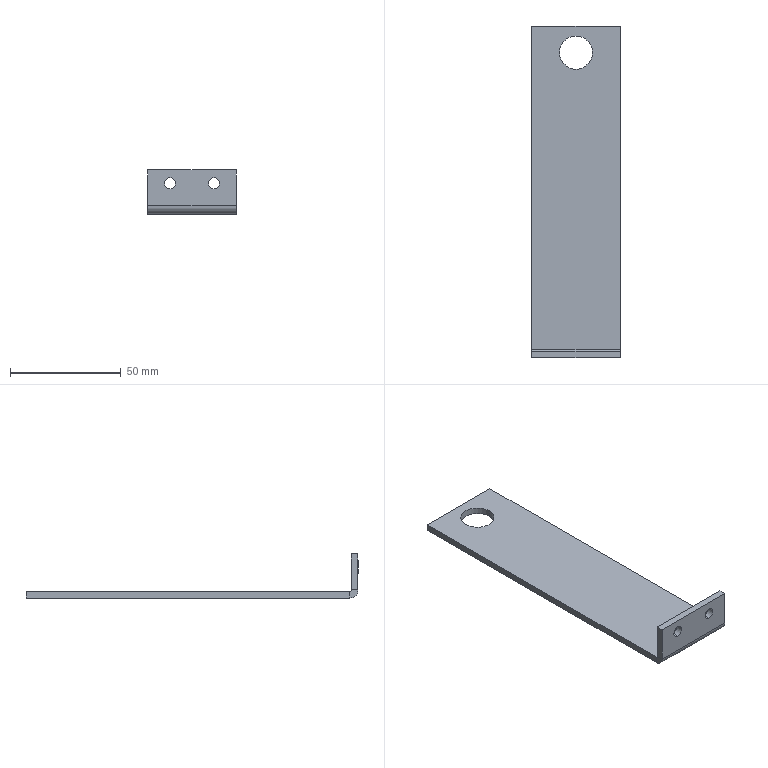Part | SolidWorks | features ICE 2, EdgeFlange 1, FlatPattern 1, SMBaseFlange 1, SheetMetal 1 | 1 solid | 20 faces | box 40 x 150 x 20 mm | volume 19277 mm3 | plane 12 | cylinder 8 | commonest cylinder face diameters 5 x4 15 x2 1.473 x1 7.473 x1
STEP:
#1=CARTESIAN_POINT('',(-10.,-75.,8.5));
#2=VERTEX_POINT('',#1);
#3=CARTESIAN_POINT('',(-10.,-75.,13.5));
#4=VERTEX_POINT('',#3);
#5=CARTESIAN_POINT('',(-10.,-75.,11.));
#6=DIRECTION('',(0.,1.,0.));
#7=DIRECTION('',(0.,0.,1.));
#8=AXIS2_PLACEMENT_3D('',#5,#6,#7);
#9=CIRCLE('',#8,2.5);
#10=EDGE_CURVE('',#2,#4,#9,.T.);
#11=ORIENTED_EDGE('',*,*,#10,.F.);
#12=CARTESIAN_POINT('',(-10.,-72.,8.5));
#13=VERTEX_POINT('',#12);
#14=CARTESIAN_POINT('',(-10.,-75.,8.5));
#15=DIRECTION('',(0.,1.,0.));
#16=VECTOR('',#15,1000.);
#17=LINE('',#14,#16);
#18=EDGE_CURVE('',#2,#13,#17,.T.);
#19=ORIENTED_EDGE('',*,*,#18,.T.);
#20=CARTESIAN_POINT('',(-10.,-72.,13.5));
#21=VERTEX_POINT('',#20);
#22=CARTESIAN_POINT('',(-10.,-72.,11.));
#23=DIRECTION('',(0.,1.,0.));
#24=DIRECTION('',(0.,0.,1.));
#25=AXIS2_PLACEMENT_3D('',#22,#23,#24);
#26=CIRCLE('',#25,2.5);
#27=EDGE_CURVE('',#13,#21,#26,.T.);
#28=ORIENTED_EDGE('',*,*,#27,.T.);
#29=CARTESIAN_POINT('',(-10.,-75.,13.5));
#30=DIRECTION('',(0.,1.,0.));
#31=VECTOR('',#30,1000.);
#32=LINE('',#29,#31);
#33=EDGE_CURVE('',#4,#21,#32,.T.);
#34=ORIENTED_EDGE('',*,*,#33,.F.);
#35=EDGE_LOOP('',(#11,#19,#28,#34));
#36=FACE_OUTER_BOUND('',#35,.T.);
#37=CARTESIAN_POINT('',(-10.,-75.,11.));
#38=DIRECTION('',(0.,1.,0.));
#39=DIRECTION('',(0.,0.,1.));
#40=AXIS2_PLACEMENT_3D('',#37,#38,#39);
#41=CYLINDRICAL_SURFACE('',#40,2.5);
#42=ADVANCED_FACE('',(#36),#41,.F.);
#43=CARTESIAN_POINT('',(10.,-75.,8.5));
#44=VERTEX_POINT('',#43);
#45=CARTESIAN_POINT('',(10.,-75.,13.5));
#46=VERTEX_POINT('',#45);
#47=CARTESIAN_POINT('',(10.,-75.,11.));
#48=DIRECTION('',(0.,1.,0.));
#49=DIRECTION('',(0.,0.,1.));
#50=AXIS2_PLACEMENT_3D('',#47,#48,#49);
#51=CIRCLE('',#50,2.5);
#52=EDGE_CURVE('',#44,#46,#51,.T.);
#53=ORIENTED_EDGE('',*,*,#52,.F.);
#54=CARTESIAN_POINT('',(10.,-72.,8.5));
#55=VERTEX_POINT('',#54);
#56=CARTESIAN_POINT('',(10.,-75.,8.5));
#57=DIRECTION('',(0.,1.,0.));
#58=VECTOR('',#57,1000.);
#59=LINE('',#56,#58);
#60=EDGE_CURVE('',#44,#55,#59,.T.);
#61=ORIENTED_EDGE('',*,*,#60,.T.);
#62=CARTESIAN_POINT('',(10.,-72.,13.5));
#63=VERTEX_POINT('',#62);
#64=CARTESIAN_POINT('',(10.,-72.,11.));
#65=DIRECTION('',(0.,1.,0.));
#66=DIRECTION('',(0.,0.,1.));
#67=AXIS2_PLACEMENT_3D('',#64,#65,#66);
#68=CIRCLE('',#67,2.5);
#69=EDGE_CURVE('',#55,#63,#68,.T.);
#70=ORIENTED_EDGE('',*,*,#69,.T.);
#71=CARTESIAN_POINT('',(10.,-75.,13.5));
#72=DIRECTION('',(0.,1.,0.));
#73=VECTOR('',#72,1000.);
#74=LINE('',#71,#73);
#75=EDGE_CURVE('',#46,#63,#74,.T.);
#76=ORIENTED_EDGE('',*,*,#75,.F.);
#77=EDGE_LOOP('',(#53,#61,#70,#76));
#78=FACE_OUTER_BOUND('',#77,.T.);
#79=CARTESIAN_POINT('',(10.,-75.,11.));
#80=DIRECTION('',(0.,1.,0.));
#81=DIRECTION('',(0.,0.,1.));
#82=AXIS2_PLACEMENT_3D('',#79,#80,#81);
#83=CYLINDRICAL_SURFACE('',#82,2.5);
#84=ADVANCED_FACE('',(#78),#83,.F.);
#85=CARTESIAN_POINT('',(-7.5,63.,-3.));
#86=VERTEX_POINT('',#85);
#87=CARTESIAN_POINT('',(7.5,63.,-3.));
#88=VERTEX_POINT('',#87);
#89=CARTESIAN_POINT('',(0.,63.,-3.));
#90=DIRECTION('',(0.,0.,1.));
#91=DIRECTION('',(1.,0.,0.));
#92=AXIS2_PLACEMENT_3D('',#89,#90,#91);
#93=CIRCLE('',#92,7.5);
#94=EDGE_CURVE('',#86,#88,#93,.T.);
#95=ORIENTED_EDGE('',*,*,#94,.F.);
#96=CARTESIAN_POINT('',(-7.5,63.,0.));
#97=VERTEX_POINT('',#96);
#98=CARTESIAN_POINT('',(-7.5,63.,-3.));
#99=DIRECTION('',(0.,0.,1.));
#100=VECTOR('',#99,1000.);
#101=LINE('',#98,#100);
#102=EDGE_CURVE('',#86,#97,#101,.T.);
#103=ORIENTED_EDGE('',*,*,#102,.T.);
#104=CARTESIAN_POINT('',(7.5,63.,0.));
#105=VERTEX_POINT('',#104);
#106=CARTESIAN_POINT('',(0.,63.,0.));
#107=DIRECTION('',(0.,0.,1.));
#108=DIRECTION('',(1.,0.,0.));
#109=AXIS2_PLACEMENT_3D('',#106,#107,#108);
#110=CIRCLE('',#109,7.5);
#111=EDGE_CURVE('',#97,#105,#110,.T.);
#112=ORIENTED_EDGE('',*,*,#111,.T.);
#113=CARTESIAN_POINT('',(7.5,63.,-3.));
#114=DIRECTION('',(0.,0.,1.));
#115=VECTOR('',#114,1000.);
#116=LINE('',#113,#115);
#117=EDGE_CURVE('',#88,#105,#116,.T.);
#118=ORIENTED_EDGE('',*,*,#117,.F.);
#119=EDGE_LOOP('',(#95,#103,#112,#118));
#120=FACE_OUTER_BOUND('',#119,.T.);
#121=CARTESIAN_POINT('',(0.,63.,-3.));
#122=DIRECTION('',(0.,0.,1.));
#123=DIRECTION('',(1.,0.,0.));
#124=AXIS2_PLACEMENT_3D('',#121,#122,#123);
#125=CYLINDRICAL_SURFACE('',#124,7.5);
#126=ADVANCED_FACE('',(#120),#125,.F.);
#127=CARTESIAN_POINT('',(20.,-71.263,0.));
#128=VERTEX_POINT('',#127);
#129=CARTESIAN_POINT('',(20.,75.,0.));
#130=VERTEX_POINT('',#129);
#131=CARTESIAN_POINT('',(20.,-75.,0.));
#132=DIRECTION('',(0.,1.,0.));
#133=VECTOR('',#132,1000.);
#134=LINE('',#131,#133);
#135=EDGE_CURVE('',#128,#130,#134,.T.);
#136=ORIENTED_EDGE('',*,*,#135,.F.);
#137=CARTESIAN_POINT('',(20.,-71.263,-3.));
#138=VERTEX_POINT('',#137);
#139=CARTESIAN_POINT('',(20.,-71.263,0.));
#140=DIRECTION('',(0.,0.,-1.));
#141=VECTOR('',#140,1000.);
#142=LINE('',#139,#141);
#143=EDGE_CURVE('',#128,#138,#142,.T.);
#144=ORIENTED_EDGE('',*,*,#143,.T.);
#145=CARTESIAN_POINT('',(20.,75.,-3.));
#146=VERTEX_POINT('',#145);
#147=CARTESIAN_POINT('',(20.,-75.,-3.));
#148=DIRECTION('',(0.,1.,0.));
#149=VECTOR('',#148,1000.);
#150=LINE('',#147,#149);
#151=EDGE_CURVE('',#138,#146,#150,.T.);
#152=ORIENTED_EDGE('',*,*,#151,.T.);
#153=CARTESIAN_POINT('',(20.,75.,-3.));
#154=DIRECTION('',(0.,0.,1.));
#155=VECTOR('',#154,1000.);
#156=LINE('',#153,#155);
#157=EDGE_CURVE('',#146,#130,#156,.T.);
#158=ORIENTED_EDGE('',*,*,#157,.T.);
#159=EDGE_LOOP('',(#136,#144,#152,#158));
#160=FACE_OUTER_BOUND('',#159,.T.);
#161=CARTESIAN_POINT('',(20.,-75.,-3.));
#162=DIRECTION('',(1.,0.,0.));
#163=DIRECTION('',(0.,0.,-1.));
#164=AXIS2_PLACEMENT_3D('',#161,#162,#163);
#165=PLANE('',#164);
#166=ADVANCED_FACE('',(#160),#165,.T.);
#167=CARTESIAN_POINT('',(0.,63.,-3.));
#168=DIRECTION('',(0.,0.,1.));
#169=DIRECTION('',(1.,0.,0.));
#170=AXIS2_PLACEMENT_3D('',#167,#168,#169);
#171=CIRCLE('',#170,7.5);
#172=EDGE_CURVE('',#88,#86,#171,.T.);
#173=ORIENTED_EDGE('',*,*,#172,.T.);
#174=ORIENTED_EDGE('',*,*,#94,.T.);
#175=EDGE_LOOP('',(#173,#174));
#176=FACE_BOUND('',#175,.T.);
#177=ORIENTED_EDGE('',*,*,#151,.F.);
#178=CARTESIAN_POINT('',(-20.,-71.263,-3.));
#179=VERTEX_POINT('',#178);
#180=CARTESIAN_POINT('',(20.,-71.263,-3.));
#181=DIRECTION('',(-1.,0.,0.));
#182=VECTOR('',#181,1000.);
#183=LINE('',#180,#182);
#184=EDGE_CURVE('',#138,#179,#183,.T.);
#185=ORIENTED_EDGE('',*,*,#184,.T.);
#186=CARTESIAN_POINT('',(-20.,75.,-3.));
#187=VERTEX_POINT('',#186);
#188=CARTESIAN_POINT('',(-20.,-75.,-3.));
#189=DIRECTION('',(0.,-1.,0.));
#190=VECTOR('',#189,1000.);
#191=LINE('',#188,#190);
#192=EDGE_CURVE('',#187,#179,#191,.T.);
#193=ORIENTED_EDGE('',*,*,#192,.F.);
#194=CARTESIAN_POINT('',(-20.,75.,-3.));
#195=DIRECTION('',(-1.,0.,0.));
#196=VECTOR('',#195,1000.);
#197=LINE('',#194,#196);
#198=EDGE_CURVE('',#146,#187,#197,.T.);
#199=ORIENTED_EDGE('',*,*,#198,.F.);
#200=EDGE_LOOP('',(#177,#185,#193,#199));
#201=FACE_OUTER_BOUND('',#200,.T.);
#202=CARTESIAN_POINT('',(0.,0.,-3.));
#203=DIRECTION('',(0.,0.,-1.));
#204=DIRECTION('',(-1.,0.,0.));
#205=AXIS2_PLACEMENT_3D('',#202,#203,#204);
#206=PLANE('',#205);
#207=ADVANCED_FACE('',(#176,#201),#206,.T.);
#208=CARTESIAN_POINT('',(0.,63.,0.));
#209=DIRECTION('',(0.,0.,1.));
#210=DIRECTION('',(1.,0.,0.));
#211=AXIS2_PLACEMENT_3D('',#208,#209,#210);
#212=CIRCLE('',#211,7.5);
#213=EDGE_CURVE('',#105,#97,#212,.T.);
#214=ORIENTED_EDGE('',*,*,#213,.F.);
#215=ORIENTED_EDGE('',*,*,#111,.F.);
#216=EDGE_LOOP('',(#214,#215));
#217=FACE_BOUND('',#216,.T.);
#218=CARTESIAN_POINT('',(-20.,-71.263,0.));
#219=VERTEX_POINT('',#218);
#220=CARTESIAN_POINT('',(20.,-71.263,0.));
#221=DIRECTION('',(-1.,0.,0.));
#222=VECTOR('',#221,1000.);
#223=LINE('',#220,#222);
#224=EDGE_CURVE('',#128,#219,#223,.T.);
#225=ORIENTED_EDGE('',*,*,#224,.F.);
#226=ORIENTED_EDGE('',*,*,#135,.T.);
#227=CARTESIAN_POINT('',(-20.,75.,0.));
#228=VERTEX_POINT('',#227);
#229=CARTESIAN_POINT('',(-20.,75.,0.));
#230=DIRECTION('',(-1.,0.,0.));
#231=VECTOR('',#230,1000.);
#232=LINE('',#229,#231);
#233=EDGE_CURVE('',#130,#228,#232,.T.);
#234=ORIENTED_EDGE('',*,*,#233,.T.);
#235=CARTESIAN_POINT('',(-20.,-75.,0.));
#236=DIRECTION('',(0.,-1.,0.));
#237=VECTOR('',#236,1000.);
#238=LINE('',#235,#237);
#239=EDGE_CURVE('',#228,#219,#238,.T.);
#240=ORIENTED_EDGE('',*,*,#239,.T.);
#241=EDGE_LOOP('',(#225,#226,#234,#240));
#242=FACE_OUTER_BOUND('',#241,.T.);
#243=CARTESIAN_POINT('',(0.,0.,0.));
#244=DIRECTION('',(0.,0.,-1.));
#245=DIRECTION('',(-1.,0.,0.));
#246=AXIS2_PLACEMENT_3D('',#243,#244,#245);
#247=PLANE('',#246);
#248=ADVANCED_FACE('',(#217,#242),#247,.F.);
#249=CARTESIAN_POINT('',(-20.,-71.263,0.));
#250=DIRECTION('',(0.,0.,-1.));
#251=VECTOR('',#250,1000.);
#252=LINE('',#249,#251);
#253=EDGE_CURVE('',#219,#179,#252,.T.);
#254=ORIENTED_EDGE('',*,*,#253,.F.);
#255=ORIENTED_EDGE('',*,*,#239,.F.);
#256=CARTESIAN_POINT('',(-20.,75.,-3.));
#257=DIRECTION('',(0.,0.,1.));
#258=VECTOR('',#257,1000.);
#259=LINE('',#256,#258);
#260=EDGE_CURVE('',#187,#228,#259,.T.);
#261=ORIENTED_EDGE('',*,*,#260,.F.);
#262=ORIENTED_EDGE('',*,*,#192,.T.);
#263=EDGE_LOOP('',(#254,#255,#261,#262));
#264=FACE_OUTER_BOUND('',#263,.T.);
#265=CARTESIAN_POINT('',(-20.,-75.,-3.));
#266=DIRECTION('',(-1.,0.,0.));
#267=DIRECTION('',(0.,0.,1.));
#268=AXIS2_PLACEMENT_3D('',#265,#266,#267);
#269=PLANE('',#268);
#270=ADVANCED_FACE('',(#264),#269,.T.);
#271=ORIENTED_EDGE('',*,*,#233,.F.);
#272=ORIENTED_EDGE('',*,*,#157,.F.);
#273=ORIENTED_EDGE('',*,*,#198,.T.);
#274=ORIENTED_EDGE('',*,*,#260,.T.);
#275=EDGE_LOOP('',(#271,#272,#273,#274));
#276=FACE_OUTER_BOUND('',#275,.T.);
#277=CARTESIAN_POINT('',(-20.,75.,-3.));
#278=DIRECTION('',(0.,1.,0.));
#279=DIRECTION('',(0.,0.,1.));
#280=AXIS2_PLACEMENT_3D('',#277,#278,#279);
#281=PLANE('',#280);
#282=ADVANCED_FACE('',(#276),#281,.T.);
#283=CARTESIAN_POINT('',(-20.,-72.,0.7366));
#284=VERTEX_POINT('',#283);
#285=CARTESIAN_POINT('',(-20.,-75.,0.7366));
#286=VERTEX_POINT('',#285);
#287=CARTESIAN_POINT('',(-20.,-75.,0.7366));
#288=DIRECTION('',(0.,-1.,0.));
#289=VECTOR('',#288,1000.);
#290=LINE('',#287,#289);
#291=EDGE_CURVE('',#284,#286,#290,.T.);
#292=ORIENTED_EDGE('',*,*,#291,.F.);
#293=CARTESIAN_POINT('',(-20.,-71.263,0.7366));
#294=DIRECTION('',(-1.,0.,0.));
#295=DIRECTION('',(0.,0.,-1.));
#296=AXIS2_PLACEMENT_3D('',#293,#294,#295);
#297=CIRCLE('',#296,0.7366);
#298=EDGE_CURVE('',#219,#284,#297,.T.);
#299=ORIENTED_EDGE('',*,*,#298,.F.);
#300=ORIENTED_EDGE('',*,*,#253,.T.);
#301=CARTESIAN_POINT('',(-20.,-71.263,0.7366));
#302=DIRECTION('',(-1.,0.,0.));
#303=DIRECTION('',(0.,0.,-1.));
#304=AXIS2_PLACEMENT_3D('',#301,#302,#303);
#305=CIRCLE('',#304,3.737);
#306=EDGE_CURVE('',#179,#286,#305,.T.);
#307=ORIENTED_EDGE('',*,*,#306,.T.);
#308=EDGE_LOOP('',(#292,#299,#300,#307));
#309=FACE_OUTER_BOUND('',#308,.T.);
#310=CARTESIAN_POINT('',(-20.,-71.263,0.7366));
#311=DIRECTION('',(-1.,0.,0.));
#312=DIRECTION('',(0.,0.,1.));
#313=AXIS2_PLACEMENT_3D('',#310,#311,#312);
#314=PLANE('',#313);
#315=ADVANCED_FACE('',(#309),#314,.T.);
#316=CARTESIAN_POINT('',(20.,-72.,0.7366));
#317=VERTEX_POINT('',#316);
#318=CARTESIAN_POINT('',(20.,-71.263,0.7366));
#319=DIRECTION('',(1.,0.,0.));
#320=DIRECTION('',(0.,0.,-1.));
#321=AXIS2_PLACEMENT_3D('',#318,#319,#320);
#322=CIRCLE('',#321,0.7366);
#323=EDGE_CURVE('',#317,#128,#322,.T.);
#324=ORIENTED_EDGE('',*,*,#323,.F.);
#325=CARTESIAN_POINT('',(20.,-75.,0.7366));
#326=VERTEX_POINT('',#325);
#327=CARTESIAN_POINT('',(20.,-72.,0.7366));
#328=DIRECTION('',(0.,-1.,0.));
#329=VECTOR('',#328,1000.);
#330=LINE('',#327,#329);
#331=EDGE_CURVE('',#317,#326,#330,.T.);
#332=ORIENTED_EDGE('',*,*,#331,.T.);
#333=CARTESIAN_POINT('',(20.,-71.263,0.7366));
#334=DIRECTION('',(1.,0.,0.));
#335=DIRECTION('',(0.,0.,-1.));
#336=AXIS2_PLACEMENT_3D('',#333,#334,#335);
#337=CIRCLE('',#336,3.737);
#338=EDGE_CURVE('',#326,#138,#337,.T.);
#339=ORIENTED_EDGE('',*,*,#338,.T.);
#340=ORIENTED_EDGE('',*,*,#143,.F.);
#341=EDGE_LOOP('',(#324,#332,#339,#340));
#342=FACE_OUTER_BOUND('',#341,.T.);
#343=CARTESIAN_POINT('',(20.,-71.263,0.7366));
#344=DIRECTION('',(-1.,0.,0.));
#345=DIRECTION('',(0.,0.,1.));
#346=AXIS2_PLACEMENT_3D('',#343,#344,#345);
#347=PLANE('',#346);
#348=ADVANCED_FACE('',(#342),#347,.F.);
#349=ORIENTED_EDGE('',*,*,#184,.F.);
#350=ORIENTED_EDGE('',*,*,#338,.F.);
#351=CARTESIAN_POINT('',(-20.,-75.,0.7366));
#352=DIRECTION('',(-1.,0.,0.));
#353=VECTOR('',#352,1000.);
#354=LINE('',#351,#353);
#355=EDGE_CURVE('',#326,#286,#354,.T.);
#356=ORIENTED_EDGE('',*,*,#355,.T.);
#357=ORIENTED_EDGE('',*,*,#306,.F.);
#358=EDGE_LOOP('',(#349,#350,#356,#357));
#359=FACE_OUTER_BOUND('',#358,.T.);
#360=CARTESIAN_POINT('',(20.,-71.263,0.7366));
#361=DIRECTION('',(1.,0.,0.));
#362=DIRECTION('',(0.,-1.,0.));
#363=AXIS2_PLACEMENT_3D('',#360,#361,#362);
#364=CYLINDRICAL_SURFACE('',#363,3.737);
#365=ADVANCED_FACE('',(#359),#364,.T.);
#366=ORIENTED_EDGE('',*,*,#224,.T.);
#367=ORIENTED_EDGE('',*,*,#298,.T.);
#368=CARTESIAN_POINT('',(-20.,-72.,0.7366));
#369=DIRECTION('',(1.,0.,0.));
#370=VECTOR('',#369,1000.);
#371=LINE('',#368,#370);
#372=EDGE_CURVE('',#284,#317,#371,.T.);
#373=ORIENTED_EDGE('',*,*,#372,.T.);
#374=ORIENTED_EDGE('',*,*,#323,.T.);
#375=EDGE_LOOP('',(#366,#367,#373,#374));
#376=FACE_OUTER_BOUND('',#375,.T.);
#377=CARTESIAN_POINT('',(20.,-71.263,0.7366));
#378=DIRECTION('',(1.,0.,0.));
#379=DIRECTION('',(0.,-1.,0.));
#380=AXIS2_PLACEMENT_3D('',#377,#378,#379);
#381=CYLINDRICAL_SURFACE('',#380,0.7366);
#382=ADVANCED_FACE('',(#376),#381,.F.);
#383=ORIENTED_EDGE('',*,*,#291,.T.);
#384=CARTESIAN_POINT('',(-20.,-75.,17.));
#385=VERTEX_POINT('',#384);
#386=CARTESIAN_POINT('',(-20.,-75.,0.));
#387=DIRECTION('',(0.,0.,-1.));
#388=VECTOR('',#387,1000.);
#389=LINE('',#386,#388);
#390=EDGE_CURVE('',#385,#286,#389,.T.);
#391=ORIENTED_EDGE('',*,*,#390,.F.);
#392=CARTESIAN_POINT('',(-20.,-72.,17.));
#393=VERTEX_POINT('',#392);
#394=CARTESIAN_POINT('',(-20.,-75.,17.));
#395=DIRECTION('',(0.,1.,0.));
#396=VECTOR('',#395,1000.);
#397=LINE('',#394,#396);
#398=EDGE_CURVE('',#385,#393,#397,.T.);
#399=ORIENTED_EDGE('',*,*,#398,.T.);
#400=CARTESIAN_POINT('',(-20.,-72.,0.));
#401=DIRECTION('',(0.,0.,-1.));
#402=VECTOR('',#401,1000.);
#403=LINE('',#400,#402);
#404=EDGE_CURVE('',#393,#284,#403,.T.);
#405=ORIENTED_EDGE('',*,*,#404,.T.);
#406=EDGE_LOOP('',(#383,#391,#399,#405));
#407=FACE_OUTER_BOUND('',#406,.T.);
#408=CARTESIAN_POINT('',(-20.,-75.,0.));
#409=DIRECTION('',(1.,0.,0.));
#410=DIRECTION('',(0.,0.,-1.));
#411=AXIS2_PLACEMENT_3D('',#408,#409,#410);
#412=PLANE('',#411);
#413=ADVANCED_FACE('',(#407),#412,.F.);
#414=ORIENTED_EDGE('',*,*,#331,.F.);
#415=CARTESIAN_POINT('',(20.,-72.,17.));
#416=VERTEX_POINT('',#415);
#417=CARTESIAN_POINT('',(20.,-72.,17.));
#418=DIRECTION('',(0.,0.,1.));
#419=VECTOR('',#418,1000.);
#420=LINE('',#417,#419);
#421=EDGE_CURVE('',#317,#416,#420,.T.);
#422=ORIENTED_EDGE('',*,*,#421,.T.);
#423=CARTESIAN_POINT('',(20.,-75.,17.));
#424=VERTEX_POINT('',#423);
#425=CARTESIAN_POINT('',(20.,-75.,17.));
#426=DIRECTION('',(0.,1.,0.));
#427=VECTOR('',#426,1000.);
#428=LINE('',#425,#427);
#429=EDGE_CURVE('',#424,#416,#428,.T.);
#430=ORIENTED_EDGE('',*,*,#429,.F.);
#431=CARTESIAN_POINT('',(20.,-75.,0.));
#432=DIRECTION('',(0.,0.,1.));
#433=VECTOR('',#432,1000.);
#434=LINE('',#431,#433);
#435=EDGE_CURVE('',#326,#424,#434,.T.);
#436=ORIENTED_EDGE('',*,*,#435,.F.);
#437=EDGE_LOOP('',(#414,#422,#430,#436));
#438=FACE_OUTER_BOUND('',#437,.T.);
#439=CARTESIAN_POINT('',(20.,-75.,17.));
#440=DIRECTION('',(-1.,0.,0.));
#441=DIRECTION('',(0.,0.,1.));
#442=AXIS2_PLACEMENT_3D('',#439,#440,#441);
#443=PLANE('',#442);
#444=ADVANCED_FACE('',(#438),#443,.F.);
#445=CARTESIAN_POINT('',(-10.,-75.,11.));
#446=DIRECTION('',(0.,1.,0.));
#447=DIRECTION('',(0.,0.,1.));
#448=AXIS2_PLACEMENT_3D('',#445,#446,#447);
#449=CIRCLE('',#448,2.5);
#450=EDGE_CURVE('',#4,#2,#449,.T.);
#451=ORIENTED_EDGE('',*,*,#450,.T.);
#452=ORIENTED_EDGE('',*,*,#10,.T.);
#453=EDGE_LOOP('',(#451,#452));
#454=FACE_BOUND('',#453,.T.);
#455=CARTESIAN_POINT('',(10.,-75.,11.));
#456=DIRECTION('',(0.,1.,0.));
#457=DIRECTION('',(0.,0.,1.));
#458=AXIS2_PLACEMENT_3D('',#455,#456,#457);
#459=CIRCLE('',#458,2.5);
#460=EDGE_CURVE('',#46,#44,#459,.T.);
#461=ORIENTED_EDGE('',*,*,#460,.T.);
#462=ORIENTED_EDGE('',*,*,#52,.T.);
#463=EDGE_LOOP('',(#461,#462));
#464=FACE_BOUND('',#463,.T.);
#465=ORIENTED_EDGE('',*,*,#355,.F.);
#466=ORIENTED_EDGE('',*,*,#435,.T.);
#467=CARTESIAN_POINT('',(0.,-75.,17.));
#468=DIRECTION('',(-1.,0.,0.));
#469=VECTOR('',#468,1000.);
#470=LINE('',#467,#469);
#471=EDGE_CURVE('',#424,#385,#470,.T.);
#472=ORIENTED_EDGE('',*,*,#471,.T.);
#473=ORIENTED_EDGE('',*,*,#390,.T.);
#474=EDGE_LOOP('',(#465,#466,#472,#473));
#475=FACE_OUTER_BOUND('',#474,.T.);
#476=CARTESIAN_POINT('',(0.,-75.,0.));
#477=DIRECTION('',(0.,1.,0.));
#478=DIRECTION('',(0.,0.,1.));
#479=AXIS2_PLACEMENT_3D('',#476,#477,#478);
#480=PLANE('',#479);
#481=ADVANCED_FACE('',(#454,#464,#475),#480,.F.);
#482=CARTESIAN_POINT('',(-10.,-72.,11.));
#483=DIRECTION('',(0.,1.,0.));
#484=DIRECTION('',(0.,0.,1.));
#485=AXIS2_PLACEMENT_3D('',#482,#483,#484);
#486=CIRCLE('',#485,2.5);
#487=EDGE_CURVE('',#21,#13,#486,.T.);
#488=ORIENTED_EDGE('',*,*,#487,.F.);
#489=ORIENTED_EDGE('',*,*,#27,.F.);
#490=EDGE_LOOP('',(#488,#489));
#491=FACE_BOUND('',#490,.T.);
#492=CARTESIAN_POINT('',(10.,-72.,11.));
#493=DIRECTION('',(0.,1.,0.));
#494=DIRECTION('',(0.,0.,1.));
#495=AXIS2_PLACEMENT_3D('',#492,#493,#494);
#496=CIRCLE('',#495,2.5);
#497=EDGE_CURVE('',#63,#55,#496,.T.);
#498=ORIENTED_EDGE('',*,*,#497,.F.);
#499=ORIENTED_EDGE('',*,*,#69,.F.);
#500=EDGE_LOOP('',(#498,#499));
#501=FACE_BOUND('',#500,.T.);
#502=ORIENTED_EDGE('',*,*,#421,.F.);
#503=ORIENTED_EDGE('',*,*,#372,.F.);
#504=ORIENTED_EDGE('',*,*,#404,.F.);
#505=CARTESIAN_POINT('',(-20.,-72.,17.));
#506=DIRECTION('',(-1.,0.,0.));
#507=VECTOR('',#506,1000.);
#508=LINE('',#505,#507);
#509=EDGE_CURVE('',#416,#393,#508,.T.);
#510=ORIENTED_EDGE('',*,*,#509,.F.);
#511=EDGE_LOOP('',(#502,#503,#504,#510));
#512=FACE_OUTER_BOUND('',#511,.T.);
#513=CARTESIAN_POINT('',(0.,-72.,0.));
#514=DIRECTION('',(0.,1.,0.));
#515=DIRECTION('',(0.,0.,1.));
#516=AXIS2_PLACEMENT_3D('',#513,#514,#515);
#517=PLANE('',#516);
#518=ADVANCED_FACE('',(#491,#501,#512),#517,.T.);
#519=ORIENTED_EDGE('',*,*,#509,.T.);
#520=ORIENTED_EDGE('',*,*,#398,.F.);
#521=ORIENTED_EDGE('',*,*,#471,.F.);
#522=ORIENTED_EDGE('',*,*,#429,.T.);
#523=EDGE_LOOP('',(#519,#520,#521,#522));
#524=FACE_OUTER_BOUND('',#523,.T.);
#525=CARTESIAN_POINT('',(-20.,-75.,17.));
#526=DIRECTION('',(0.,0.,-1.));
#527=DIRECTION('',(0.,1.,0.));
#528=AXIS2_PLACEMENT_3D('',#525,#526,#527);
#529=PLANE('',#528);
#530=ADVANCED_FACE('',(#524),#529,.F.);
#531=ORIENTED_EDGE('',*,*,#102,.F.);
#532=ORIENTED_EDGE('',*,*,#172,.F.);
#533=ORIENTED_EDGE('',*,*,#117,.T.);
#534=ORIENTED_EDGE('',*,*,#213,.T.);
#535=EDGE_LOOP('',(#531,#532,#533,#534));
#536=FACE_OUTER_BOUND('',#535,.T.);
#537=CARTESIAN_POINT('',(0.,63.,-3.));
#538=DIRECTION('',(0.,0.,1.));
#539=DIRECTION('',(1.,0.,0.));
#540=AXIS2_PLACEMENT_3D('',#537,#538,#539);
#541=CYLINDRICAL_SURFACE('',#540,7.5);
#542=ADVANCED_FACE('',(#536),#541,.F.);
#543=ORIENTED_EDGE('',*,*,#60,.F.);
#544=ORIENTED_EDGE('',*,*,#460,.F.);
#545=ORIENTED_EDGE('',*,*,#75,.T.);
#546=ORIENTED_EDGE('',*,*,#497,.T.);
#547=EDGE_LOOP('',(#543,#544,#545,#546));
#548=FACE_OUTER_BOUND('',#547,.T.);
#549=CARTESIAN_POINT('',(10.,-75.,11.));
#550=DIRECTION('',(0.,1.,0.));
#551=DIRECTION('',(0.,0.,1.));
#552=AXIS2_PLACEMENT_3D('',#549,#550,#551);
#553=CYLINDRICAL_SURFACE('',#552,2.5);
#554=ADVANCED_FACE('',(#548),#553,.F.);
#555=ORIENTED_EDGE('',*,*,#18,.F.);
#556=ORIENTED_EDGE('',*,*,#450,.F.);
#557=ORIENTED_EDGE('',*,*,#33,.T.);
#558=ORIENTED_EDGE('',*,*,#487,.T.);
#559=EDGE_LOOP('',(#555,#556,#557,#558));
#560=FACE_OUTER_BOUND('',#559,.T.);
#561=CARTESIAN_POINT('',(-10.,-75.,11.));
#562=DIRECTION('',(0.,1.,0.));
#563=DIRECTION('',(0.,0.,1.));
#564=AXIS2_PLACEMENT_3D('',#561,#562,#563);
#565=CYLINDRICAL_SURFACE('',#564,2.5);
#566=ADVANCED_FACE('',(#560),#565,.F.);
#567=CLOSED_SHELL('',(#42,#84,#126,#166,#207,#248,#270,#282,#315,#348,#365,#382,#413,#444,#481,#518,#530,#542,#554,#566));
#568=MANIFOLD_SOLID_BREP('',#567);
#569=CARTESIAN_POINT('',(0.,0.,0.));
#570=DIRECTION('',(0.,0.,1.));
#571=DIRECTION('',(1.,0.,0.));
#572=AXIS2_PLACEMENT_3D('',#569,#570,#571);
#573=(LENGTH_UNIT()NAMED_UNIT(*)SI_UNIT(.MILLI.,.METRE.));
#574=UNCERTAINTY_MEASURE_WITH_UNIT(LENGTH_MEASURE(0.00001),#573,'','');
#575=(NAMED_UNIT(*)PLANE_ANGLE_UNIT()SI_UNIT($,.RADIAN.));
#576=(NAMED_UNIT(*)SI_UNIT($,.STERADIAN.)SOLID_ANGLE_UNIT());
#577=(GEOMETRIC_REPRESENTATION_CONTEXT(3)GLOBAL_UNCERTAINTY_ASSIGNED_CONTEXT((#574))GLOBAL_UNIT_ASSIGNED_CONTEXT((#573,#575,#576))REPRESENTATION_CONTEXT('',''));
#578=ADVANCED_BREP_SHAPE_REPRESENTATION('',(#568,#572),#577);